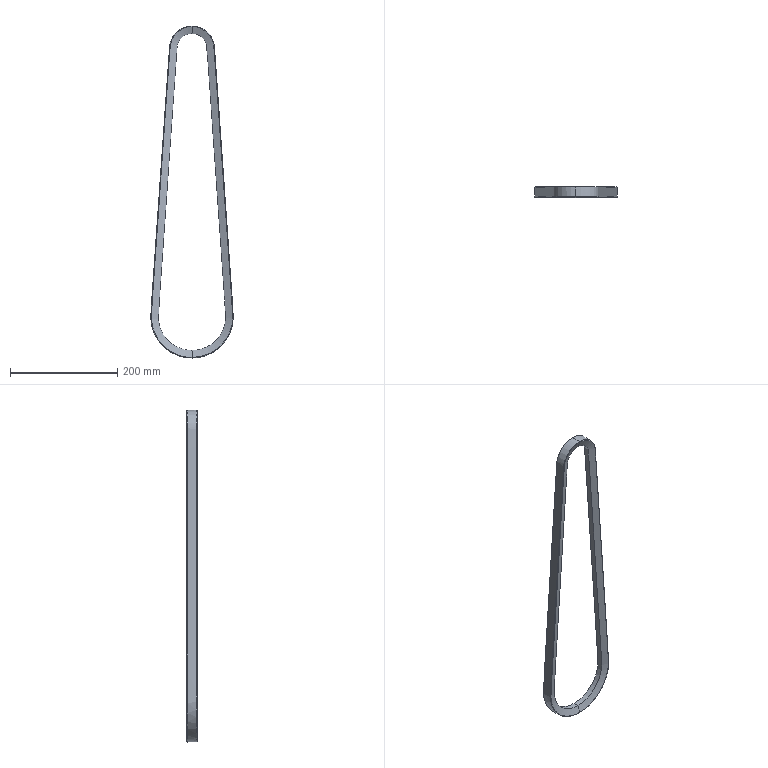Part | STEP file | Tube feed_id146_x_t | 1 solid | 12 faces | box 153.999 x 19.507 x 619 mm | volume 281240 mm3 | spline 12